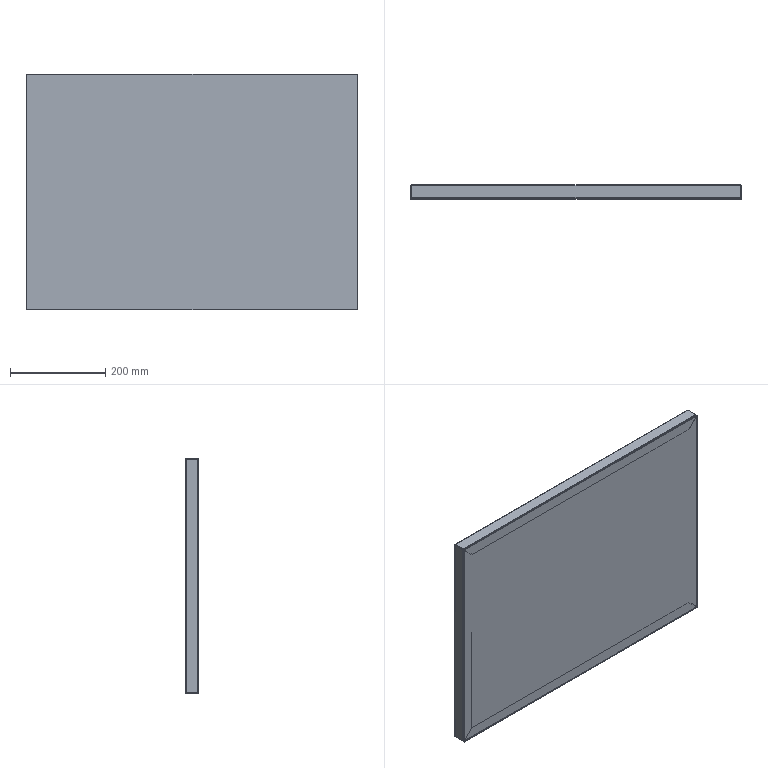Part | SolidWorks | features EdgeFlange 2, FlatPattern 1, HoleWzd 1, ICE 1, SMBaseFlange 1, SheetMetal 1 | 1 solid | 84 faces | box 696 x 29.2 x 496 mm | volume 963992 mm3 | plane 40 | cylinder 28 | spline 16 | commonest cylinder face diameters 7 x12 2 x8 4.4 x8